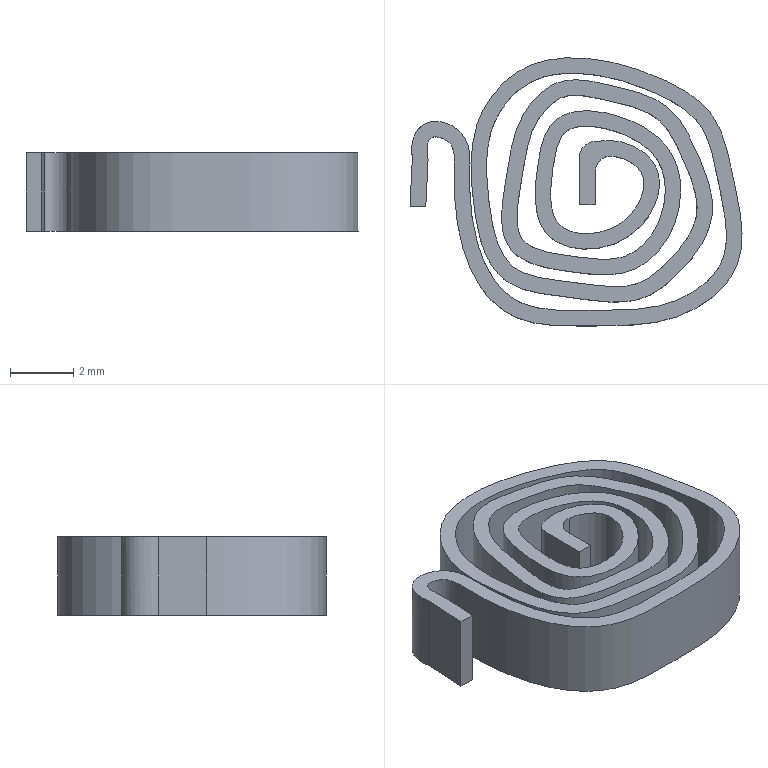Part | SolidWorks | features ICE 3, Fillet 2, Scale 1, Sweep 1 | 1 solid | 12 faces | box 10.516 x 8.505 x 2.5 mm | volume 95.086 mm3 | plane 8 | spline 2 | cylinder 2 | commonest cylinder face diameters 1 x2